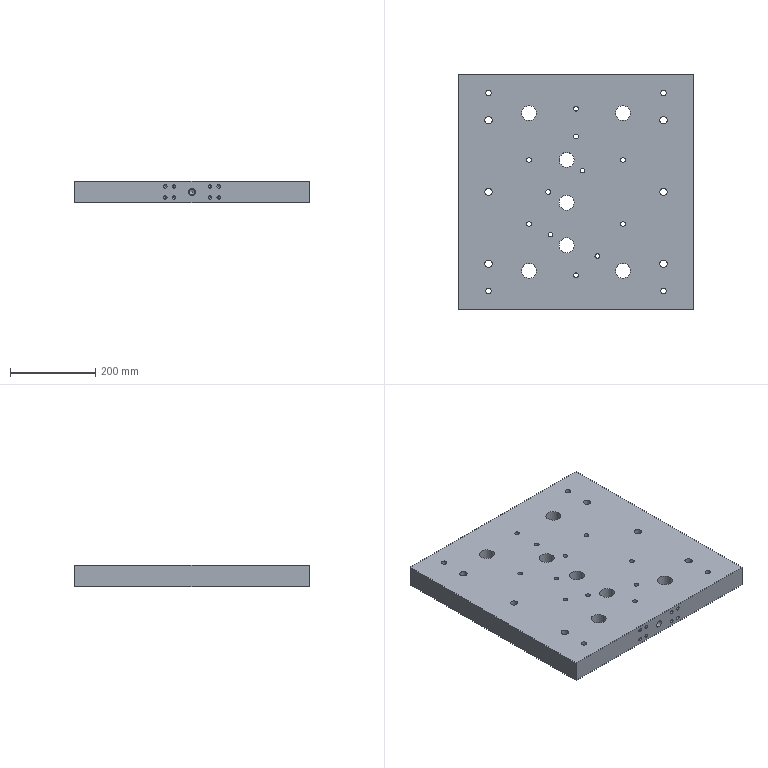Part | STEP file | 车灯-后视镜_id466_x_t | 1 solid | 204 faces | box 550 x 550 x 50 mm | volume 14539056 mm3 | cylinder 113 | plane 57 | cone 34 | commonest cylinder face diameters 8 x32 6.9 x24 17 x17 11 x11 35 x7 25 x6